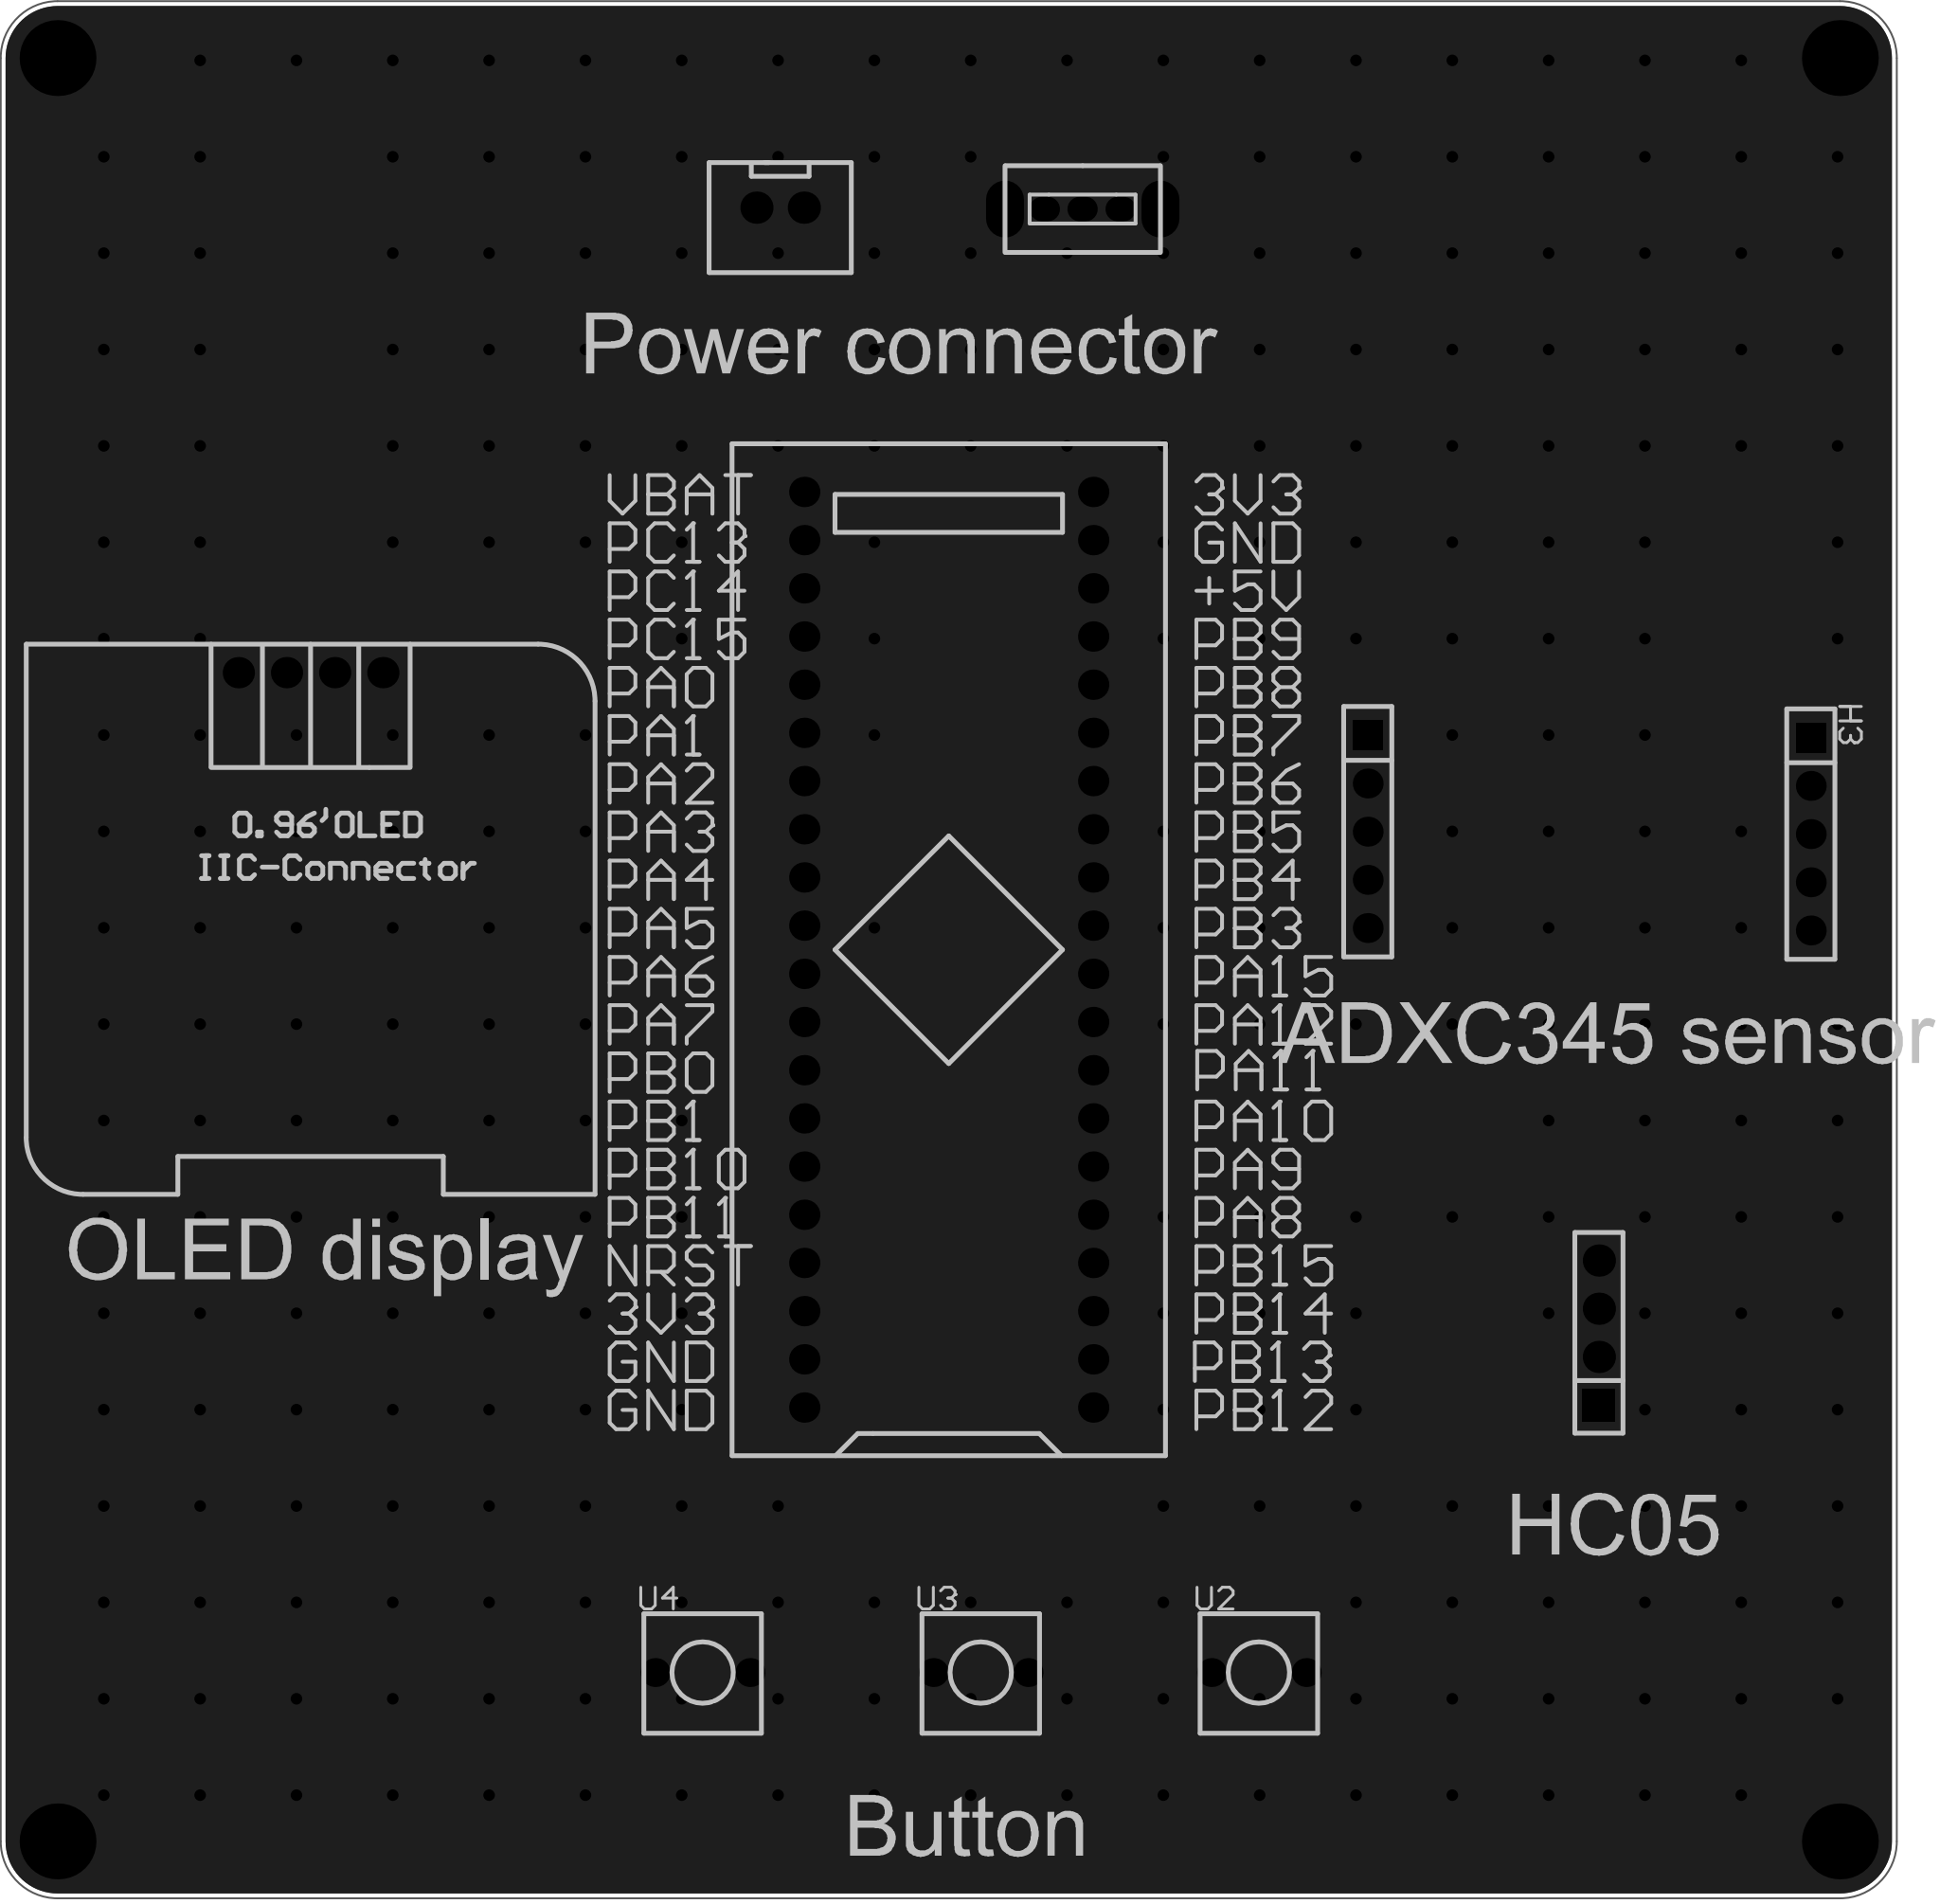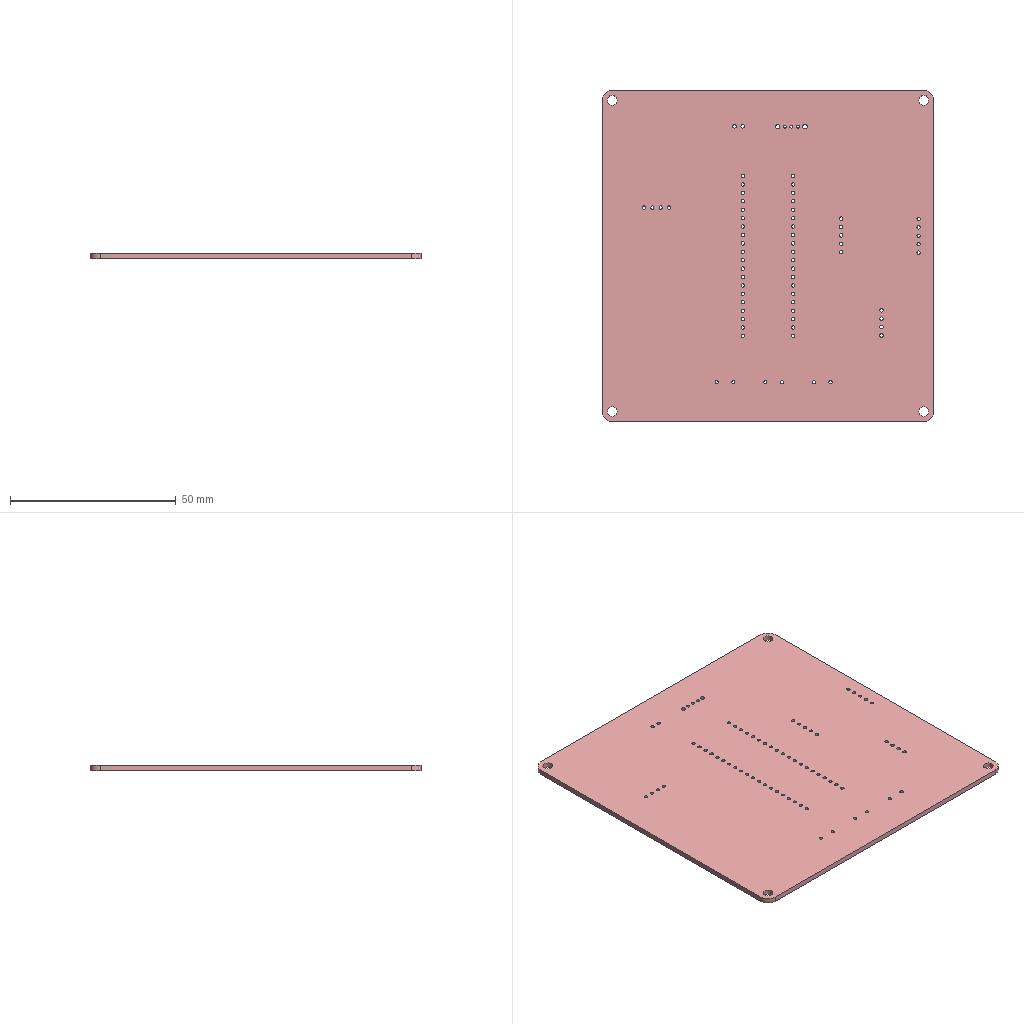Circuit board layout | Altium Designer | box 100 x 100 x 1.6 mm
Layer stack:
# Altium Designer layer stack of  (unit mm; dielectric type: 0 none, 1 core, 2 prepreg, 3 surface material)
index,name,kind,layer,copper_thickness_mm,dielectric_type,dielectric_thickness_mm,dielectric_material,dielectric_constant
0,Top Paste Mask Layer,other,,,,,,
1,Top Silkscreen Layer,other,,,,,,
2,Top Solder Mask Layer,dielectric,,,3,0.01,,3.3
3,Top Layer,copper,Top Layer,0.035,,,,
4,Dielectric1,dielectric,,,3,1.51,FR4,4.5
5,Bottom Layer,copper,Bottom Layer,0.035,,,,
6,Bottom Solder Mask Layer,dielectric,,,3,0.01,,3.3
7,Bottom Silkscreen Layer,other,,,,,,
8,Bottom Paste Mask Layer,other,,,,,,
# drill layer pairs: low layer,high layer
drill_pair,Top Layer,Bottom Layer
Part placement:
Designator,Comment,Layer,Footprint,Center-X(mm),Center-Y(mm),Rotation
U1,STM32F103C8T6-Card,TopLayer,CONN-TH_L53.3-W22.9_STM32F103C8T6-CARD,141.351,130.937,90
OLED1,,TopLayer,0.96OLED_4P,107.696,145.542,0
CN4,XH2.54*2P_through-hole,TopLayer,CONN-TH_2P-P2.50-XH2.54-2P,132.461,170.053,0
SW5,,TopLayer,拨动开关,148.417,169.978,0
H2,,TopLayer,HDR-TH_4P-P2.54-V-F,175.641,110.744,90
H3,,TopLayer,HDR-TH_5P-P2.54-V-F,186.817,137.033,270
H1,,TopLayer,HDR-TH_5P-P2.54-V-F,163.449,137.16,270
U2,TL59BF160Q,TopLayer,KEY-TH_L6.2-W6.2-P5.00,157.707,92.837,0
U3,TL59BF160Q,TopLayer,KEY-TH_L6.2-W6.2-P5.00,143.038,92.837,0
U4,TL59BF160Q,TopLayer,KEY-TH_L6.2-W6.2-P5.00,128.37,92.837,0
Pad and via stacks:
# Altium Designer via and pad stacks of  (unit mm). Each distinct definition once, with the count of objects using it.
# via: kind,start_layer,end_layer,hole_mm,diameter_mm,mode(0 simple;1 top-mid-bottom;2 full stack),diameter_per_layer,count,example_net
# pad: kind,layer,hole_mm,hole_type(0 round;1 square;2 slot),plating,top_size,top_shape(1 round;2 rect;3 octagon;9 rounded rect),mid_size,bottom_size,mode,footprint,size_per_layer,count,example
pad,Multi-Layer,3,0,plated,4x4,1,4x4,4x4,0,,,4,1
pad,Multi-Layer,1,0,plated,1.6x1.6,1,1.6x1.6,1.6x1.6,0,CONN-TH_L53.3-W22.9_STM32F103C8T6-CARD,,40,U1.1
pad,Multi-Layer,1,0,plated,1.65x1.65,1,1.65x1.65,1.65x1.65,0,0.96OLED_4P,,4,OLED1.4
pad,Multi-Layer,1.05,0,plated,1.7x1.7,1,1.7x1.7,1.7x1.7,0,CONN-TH_2P-P2.50-XH2.54-2P,,2,CN4.2
pad,Multi-Layer,0.8992,0,plated,1.6x1.3,1,1.6x1.3,1.6x1.3,0,\u00B2\u00A6\u00B6\u00AF\u00BF\u00AA\u00B9\u00D8,,3,SW5.1
pad,Multi-Layer,1.3,0,plated,3x1.999,1,3x1.999,3x1.999,0,\u00B2\u00A6\u00B6\u00AF\u00BF\u00AA\u00B9\u00D8,,2,SW5.4
pad,Multi-Layer,1.1,0,plated,1.7x1.7,2,1.7x1.7,1.7x1.7,0,HDR-TH_4P-P2.54-V-F,,1,H2.1
pad,Multi-Layer,1.1,0,plated,1.7x1.7,1,1.7x1.7,1.7x1.7,0,HDR-TH_4P-P2.54-V-F,,3,H2.2
pad,Multi-Layer,1.02,0,plated,1.575x1.575,1,1.575x1.575,1.575x1.575,0,HDR-TH_5P-P2.54-V-F,,8,H3.5
pad,Multi-Layer,1.02,0,plated,1.575x1.575,2,1.575x1.575,1.575x1.575,0,HDR-TH_5P-P2.54-V-F,,2,H3.1
pad,Multi-Layer,1,0,plated,1.524x1.524,1,1.524x1.524,1.524x1.524,0,KEY-TH_L6.2-W6.2-P5.00,,6,U2.2
via,Top Layer,Bottom Layer,0.3048,0.61,0,,286,GND
Copper pours:
name,layer,net,type(0 solid;1 hatched;2 none)
Bottom Layer-GND,Bottom Layer,GND,0
Top Layer-GND,Top Layer,GND,0
Design rules, without the lines most boards share:
# Altium Designer design rules of  (exported by Altium Designer, unit mm)
# columns: name | kind | enabled | priority | scope1 | scope2 | descriptor | typed fields (field=value)
Copper_copperRegion_copperThickness1oz | 0 | disabled | 4 | All | All | Clearance Constraint (Gap=5.984mil) (Disabled)(All),(All) | gap=0.152
Copper_copperRegion_copperThickness1oz_1 | 63 | disabled | 4 | All | All | Board Clearance Constraint (Gap=0mil) (Disabled)(All) |
Copper_copperRegion_Copper_copperRegion | 0 | disabled | 5 | All | All | Clearance Constraint (Gap=5.984mil) (Disabled)(All),(All) | gap=0.152
Copper_copperRegion_Copper_copperRegion_1 | 63 | disabled | 5 | All | All | Board Clearance Constraint (Gap=0mil) (Disabled)(All) |
copperThickness1oz | 0 | enabled | 6 | All | All | Clearance Constraint (Gap=5.984mil) (All),(All) | gap=0.152
copperThickness1oz_1 | 63 | enabled | 6 | All | All | Board Clearance Constraint (Gap=0mil) (All) |
copperRegion_copperThickness1oz | 20 | disabled | 1 | All | All | Polygon Connect Rule(Relief Connect )(Conductor Width=10mil) (Relief Angle=90 Angle) (Entries=4) (Air Gap Width=10mil) (Disabled)(All),(All) | connect_style(0=relief,1=direct,2=none)=0 relief_conductor_width=0.254 relief_entries=4
copperRegion_Copper_copperRegion | 20 | disabled | 2 | All | All | Polygon Connect Rule(Relief Connect )(Conductor Width=10mil) (Relief Angle=90 Angle) (Entries=4) (Air Gap Width=10mil) (Disabled)(All),(All) | connect_style(0=relief,1=direct,2=none)=0 relief_conductor_width=0.254 relief_entries=4
copperRegion | 20 | enabled | 3 | All | All | Polygon Connect Rule(Relief Connect )(Conductor Width=10mil) (Relief Angle=90 Angle) (Entries=4) (Air Gap Width=10mil) (All),(All) | connect_style(0=relief,1=direct,2=none)=0 relief_conductor_width=0.254 relief_entries=4